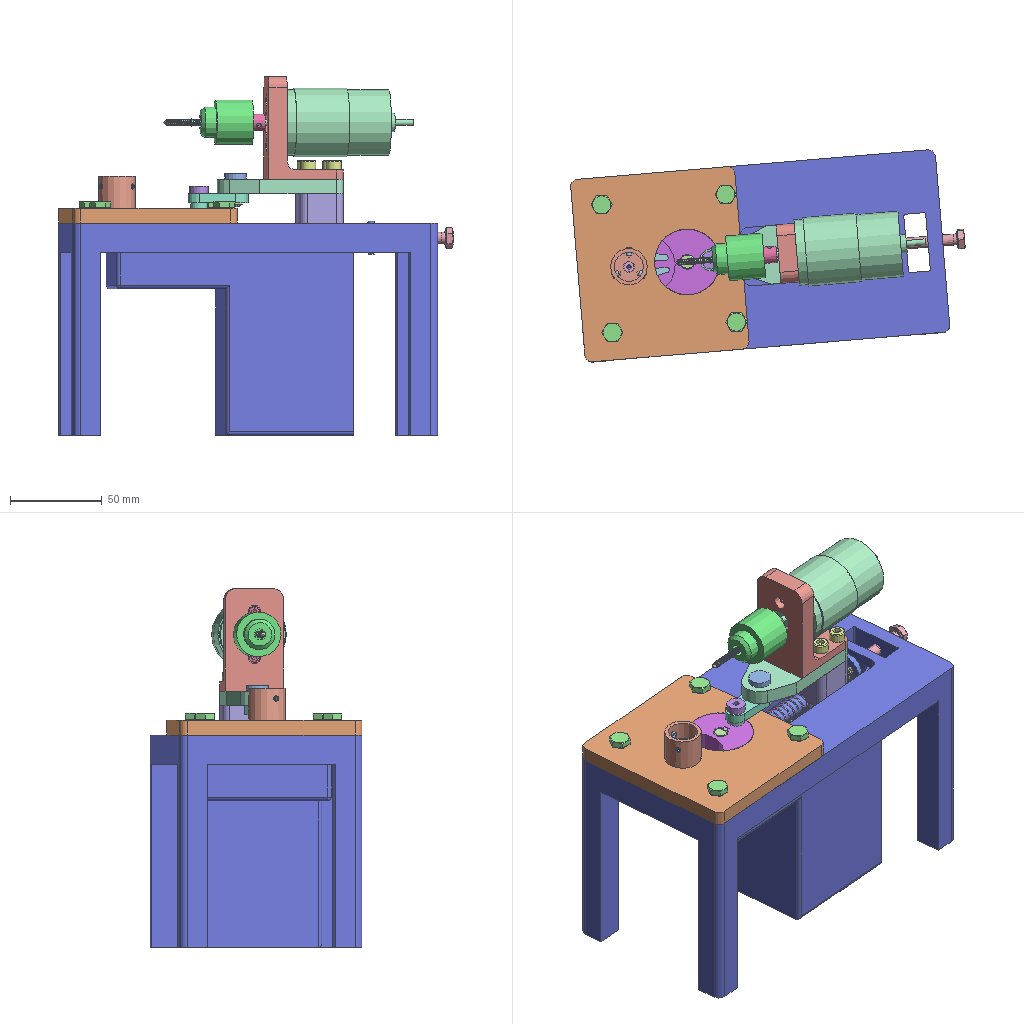Assembly | NX | 52 different items | 66 placed | box 216 x 116 x 196 mm
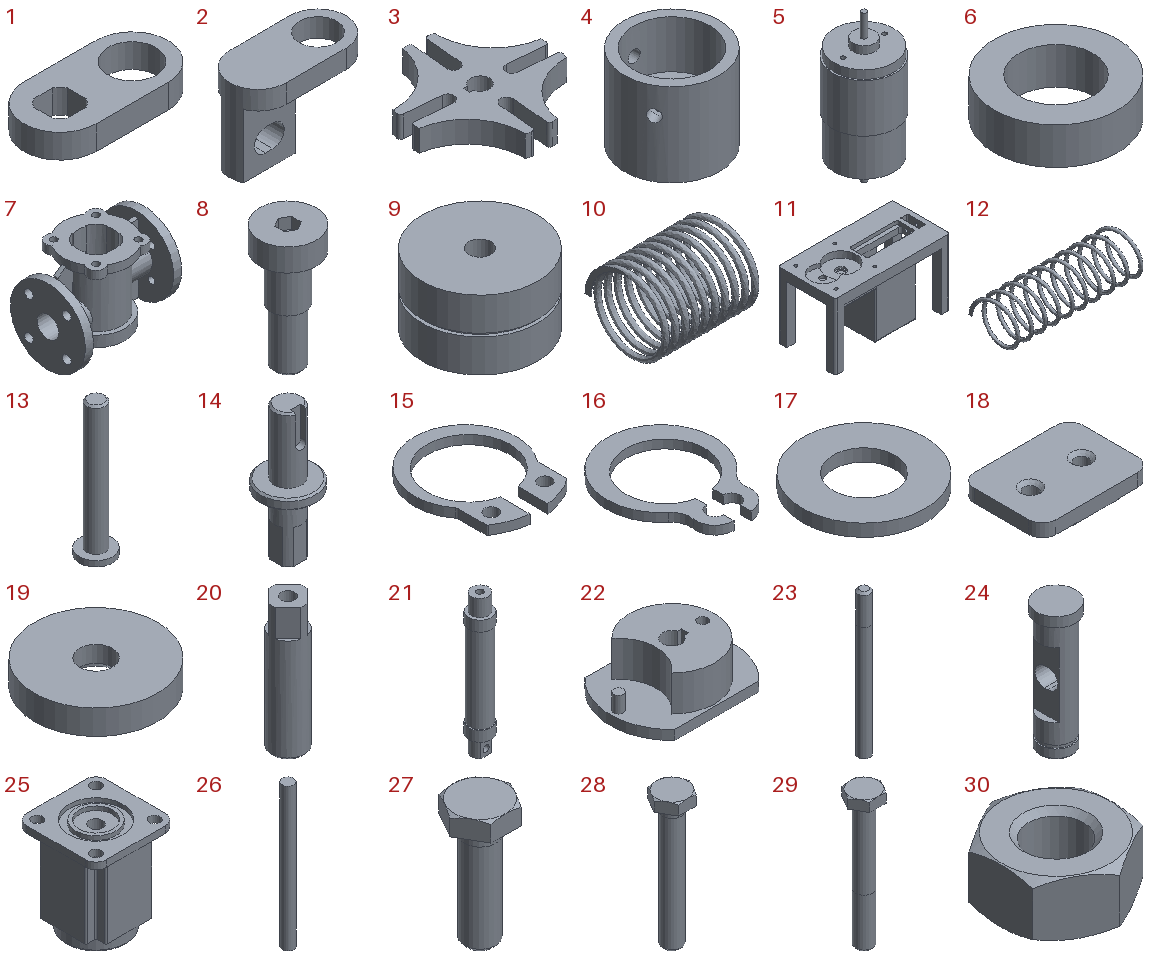Parts list (item | quantity | size | volume | features):
1 | x1 | 30 x 15 x 5 mm | 1391 mm3 | features BREP 1, DATUM_CSYS 1
2 | x1 | 31 x 15 x 22 mm | 2937 mm3 | features BREP 1, DATUM_CSYS 1
3 | x1 | 43.943 x 43.943 x 10.8 mm | 5233 mm3 | features BREP 1, DATUM_CSYS 1
4 | x1 | 20 x 20 x 17.5 mm | 3306 mm3 | features BREP 1, DATUM_CSYS 1
5 | x1 | 37.5 x 37.5 x 88.5 mm | 61229 mm3 | features BREP 1, DATUM_CSYS 1
6 | x1 | 10 x 10 x 3 mm | 150.796 mm3 | features BREP 1, DATUM_CSYS 1
7 | x1 | 180 x 140 x 175 mm | 1165814 mm3 | features DATUM_CSYS 16, SKETCH 15, EXTRUDE 12, SWP104 7, UNITE 3, PULL_FACE 1
8 | x1 | 10 x 10 x 21.75 mm | 714.374 mm3 | features BREP 1, DATUM_CSYS 1
9 | x1 | 35 x 35 x 21 mm | 19346 mm3 | features BREP 1, DATUM_CSYS 1
10 | x1 | 15 x 11.8 x 11.8 mm | 171.601 mm3 | features BREP 1, DATUM_CSYS 1
11 | x1 | 200 x 100 x 116 mm | 451086 mm3 | features EXTRUDE 14, DATUM_CSYS 8, SKETCH 7, BLEND 4, BREP 1, SHELL 1, UNITE 1
12 | x1 | 37 x 11.8 x 11.8 mm | 173.342 mm3 | features BREP 1, DATUM_CSYS 1
13 | x1 | 18 x 18 x 73 mm | 5726 mm3 | features BREP 1, DATUM_CSYS 1
14 | x1 | 16 x 16 x 39 mm | 2221 mm3 | features DATUM_CSYS 2, EXTRUDE 2, BREP 1, SKETCH 1
15 | x1 | 11.5 x 13.997 x 1 mm | 50.713 mm3 | features BREP 1, DATUM_CSYS 1
16 | x1 | 7.6 x 9.565 x 0.6 mm | 14.427 mm3 | features BREP 1, DATUM_CSYS 1
17 | x1 | 20 x 20 x 2 mm | 471.239 mm3 | features BREP 1, DATUM_CSYS 1
18 | x1 | 32 x 24 x 4 mm | 2844 mm3 | features BREP 1, DATUM_CSYS 1
19 | x2 | 15 x 15 x 3 mm | 485.114 mm3 | features BREP 1, DATUM_CSYS 1
20 | x1 | 6 x 6 x 24 mm | 581.313 mm3 | features BREP 1
21 | x1 | 22 x 22 x 134 mm | 36167 mm3 | features BREP 1, DATUM_CSYS 1
22 | x1 | 52 x 38 x 19 mm | 18337 mm3 | features BREP 1, DATUM_CSYS 1
23 | x1 | 6 x 6 x 72 mm | 2027 mm3 | features BREP 1, DATUM_CSYS 1
24 | x1 | 12 x 12 x 39 mm | 2499 mm3 | features BREP 1, DATUM_CSYS 1
25 | x1 | 60 x 60 x 70 mm | 149838 mm3 | features DATUM_CSYS 8, EXTRUDE 8, SKETCH 7, BLEND 2
26 | x1 | 8 x 8 x 100 mm | 5027 mm3 | features BREP 1, DATUM_CSYS 1
27 | x4 | 11.547 x 10 x 24 mm | 891.515 mm3 | features BREP 1, DATUM_CSYS 1
28 | x1 | 11.547 x 10 x 44 mm | 1457 mm3 | features BREP 1, DATUM_CSYS 1
29 | x1 | 11.547 x 10 x 49 mm | 1599 mm3 | features BREP 1, DATUM_CSYS 1
30 | x1 | 10 x 11.547 x 5 mm | 327.462 mm3 | features BREP 1, DATUM_CSYS 1
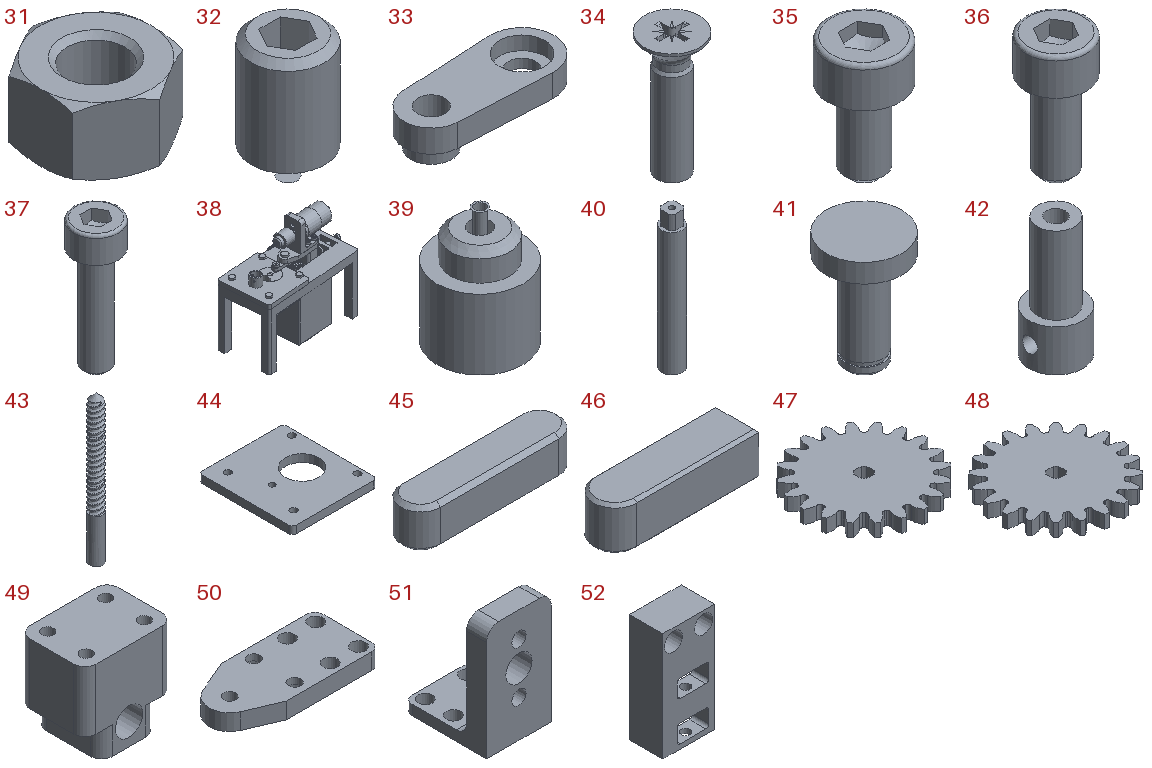31 | x1 | 13 x 15.011 x 7.9 mm | 859.913 mm3 | features BREP 1, DATUM_CSYS 1
32 | x3 | 3 x 3 x 5 mm | 26.266 mm3 | features BREP 1, DATUM_CSYS 1
33 | x1 | 33 x 14 x 8 mm | 1642 mm3 | features BREP 1, DATUM_CSYS 1
34 | x5 | 5.5 x 5.5 x 12.001 mm | 94.702 mm3 | features BREP 1, DATUM_CSYS 1
35 | x2 | 5.5 x 5.5 x 9 mm | 106.3 mm3 | features BREP 1, DATUM_CSYS 1
36 | x1 | 8.5 x 8.5 x 17 mm | 479.07 mm3 | features BREP 1, DATUM_CSYS 1
37 | x4 | 8.5 x 8.5 x 25 mm | 636.149 mm3 | features BREP 1, DATUM_CSYS 1
38 | x1 | 215.544 x 115.774 x 196 mm | 881623 mm3 | features BREP 72, DATUM_CSYS 56, META 40, EXTRUDE 29, SKETCH 21, BLEND 6, CYLINDER 2, FSET 2, SHELL 1, UNITE 1
39 | x1 | 24.5 x 24.5 x 33 mm | 10618 mm3 | features BREP 1, DATUM_CSYS 1
40 | x1 | 10 x 10 x 67 mm | 4993 mm3 | features DATUM_CSYS 4, EXTRUDE 3, SKETCH 3
41 | x1 | 12 x 12 x 18 mm | 758.995 mm3 | features BREP 1, DATUM_CSYS 1
42 | x1 | 9 x 9 x 20 mm | 655.524 mm3 | features BREP 1, DATUM_CSYS 1
43 | x1 | 3 x 3.001 x 33.5 mm | 185.13 mm3 | features BREP 1, DATUM_CSYS 1
44 | x1 | 90 x 100 x 8 mm | 62289 mm3 | features BREP 1, DATUM_CSYS 1
45 | x1 | 8 x 2 x 2 mm | 29.569 mm3 | features BREP 1, DATUM_CSYS 1
46 | x1 | 10 x 3 x 3 mm | 86.133 mm3 | features BREP 1, DATUM_CSYS 1
47 | x1 | 66 x 66 x 7 mm | 19139 mm3 | features BREP 20, META 20, DATUM_CSYS 3, SKETCH 2, CYLINDER 1, EXTRUDE 1, FSET 1
48 | x1 | 65.481 x 65.481 x 7 mm | 19139 mm3 | features BREP 20, META 20, DATUM_CSYS 2, CYLINDER 1, EXTRUDE 1, FSET 1, SKETCH 1
49 | x1 | 32 x 24 x 32 mm | 18240 mm3 | features BREP 1, DATUM_CSYS 1
50 | x1 | 68 x 32 x 8 mm | 13164 mm3 | features BREP 1, DATUM_CSYS 1
51 | x1 | 32 x 41 x 56 mm | 19804 mm3 | features BREP 1, DATUM_CSYS 1
52 | x1 | - | 28457 mm3 | features BREP 1, DATUM_CSYS 1
Mates (type | each side: item.copy, entity, surface, feature):
Concentric | 22.1 edge | 11.1 edge
Concentric | 3.1 edge | 11.1 edge
Concentric | 14.1 edge | 22.1 edge
AlignLock | 14.1 edge | 22.1 edge
Concentric | 51.1 edge | 50.1 edge
Concentric | 50.1 edge | 51.1 edge
Concentric | 5.1 edge | 51.1 edge | 2 times
Concentric | 42.1 edge | 5.1 edge
Concentric | 39.1 edge | 42.1 edge
Concentric | 43.1 edge | 39.1 edge
Concentric | 37.1 edge | 51.1 edge | 4 times
Concentric | 49.1 edge | 50.1 edge | 2 times
Concentric | 41.1 edge | 50.1 edge
Concentric | 6.1 edge | 33.1 edge
Concentric | 6.1 edge | 50.1 edge
Concentric | 8.1 edge | 33.1 edge
Concentric | 16.1 edge | 41.1 edge
Concentric | 33.1 edge | 22.1 edge
AlignLock | 49.1 face cylinder Body(1) | 11.1 face cylinder Body(1)
AlignLock | 13.1 face cylinder Body(1) | 49.1 face cylinder Body(1)
Concentric | 18.1 edge | 49.1 edge | 2 times
Concentric | 34.1 edge | 18.1 edge | 2 times
Concentric | 28.1 edge | 13.1 edge
AlignLock | 32.1 face cylinder Body(1) | 4.1 face cylinder Body(1) | 3 times
Distance | 32.1 edge | 4.1 face cylinder Body(1) | 3 times
Touch | 46.1 face plane Body(1) | 22.1 face plane Body(1) | 2 times
AlignLock | 46.1 edge | 22.1 edge
Concentric | 35.1 edge | 51.1 edge | 2 times
Touch | 45.1 face plane Body(1) | 20.1 face plane Body(1) | 2 times
Touch | 45.1 face cylinder Body(1) | 20.1 face cylinder Body(1)
Concentric | 20.1 edge | 3.1 edge
Perpendicular | 45.1 face plane Body(1) | 3.1 face plane Body(1)
Concentric | 44.1 edge | 11.1 edge
AlignLock | 44.1 edge | 11.1 edge
Concentric | 27.1 edge | 44.1 edge | 4 times
AlignLock | 4.1 face cylinder Body(1) | 20.1 face cylinder Body(1)
Touch | 4.1 face plane Body(1) | 44.1 face plane Body(1)
Concentric | 34.1 edge | 4.1 edge
Concentric | 34.1 edge | 19.1 edge | 2 times
Concentric | 19.1 edge | 14.1 edge
Concentric | 47.1 edge | 14.1 edge
Concentric | 19.1 edge | 40.1 edge
Concentric | 25.1 edge | 40.1 edge
Concentric | 48.1 edge | 40.1 edge
AlignLock | 40.1 edge | 48.1 edge